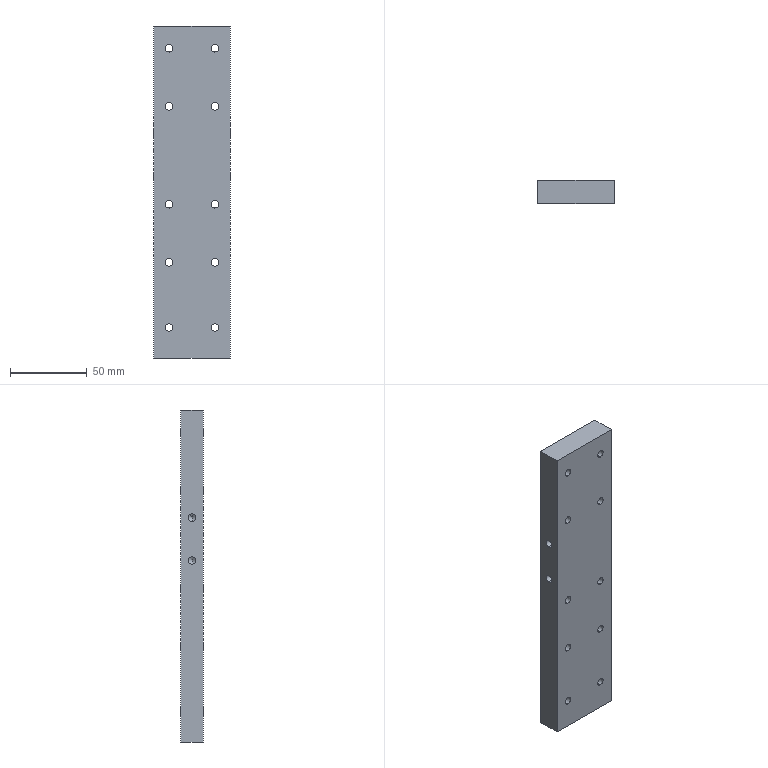Part | 1 solid | 50 faces | box 50 x 15 x 217 mm | volume 157448 mm3 | cylinder 32 | cone 12 | plane 6 | commonest cylinder face diameters 5 x28 6.8 x4
STEP:
#1=CARTESIAN_POINT('',(-11.6,7.5,-93.5));
#2=VERTEX_POINT('',#1);
#3=CARTESIAN_POINT('',(-18.4,7.5,-93.5));
#4=VERTEX_POINT('',#3);
#5=CARTESIAN_POINT('',(-15.,7.5,-93.5));
#6=DIRECTION('',(0.,0.,-1.));
#7=DIRECTION('',(-1.,0.,0.));
#8=AXIS2_PLACEMENT_3D('',#5,#6,#7);
#9=CIRCLE('',#8,3.4);
#10=EDGE_CURVE('',#2,#4,#9,.T.);
#11=ORIENTED_EDGE('',*,*,#10,.F.);
#12=CARTESIAN_POINT('',(-11.6,7.5,-108.5));
#13=VERTEX_POINT('',#12);
#14=CARTESIAN_POINT('',(-11.6,7.5,-108.5));
#15=DIRECTION('',(0.,0.,-1.));
#16=VECTOR('',#15,1000.);
#17=LINE('',#14,#16);
#18=EDGE_CURVE('',#2,#13,#17,.T.);
#19=ORIENTED_EDGE('',*,*,#18,.T.);
#20=CARTESIAN_POINT('',(-18.4,7.5,-108.5));
#21=VERTEX_POINT('',#20);
#22=CARTESIAN_POINT('',(-15.,7.5,-108.5));
#23=DIRECTION('',(0.,0.,-1.));
#24=DIRECTION('',(-1.,0.,0.));
#25=AXIS2_PLACEMENT_3D('',#22,#23,#24);
#26=CIRCLE('',#25,3.4);
#27=EDGE_CURVE('',#13,#21,#26,.T.);
#28=ORIENTED_EDGE('',*,*,#27,.T.);
#29=CARTESIAN_POINT('',(-18.4,7.5,-108.5));
#30=DIRECTION('',(0.,0.,-1.));
#31=VECTOR('',#30,1000.);
#32=LINE('',#29,#31);
#33=EDGE_CURVE('',#4,#21,#32,.T.);
#34=ORIENTED_EDGE('',*,*,#33,.F.);
#35=EDGE_LOOP('',(#11,#19,#28,#34));
#36=FACE_OUTER_BOUND('',#35,.T.);
#37=CARTESIAN_POINT('',(-15.,7.5,-108.5));
#38=DIRECTION('',(0.,0.,-1.));
#39=DIRECTION('',(-1.,0.,0.));
#40=AXIS2_PLACEMENT_3D('',#37,#38,#39);
#41=CYLINDRICAL_SURFACE('',#40,3.4);
#42=ADVANCED_FACE('',(#36),#41,.F.);
#43=CARTESIAN_POINT('',(-15.,7.5,-91.457));
#44=VERTEX_POINT('',#43);
#45=CARTESIAN_POINT('',(-18.4,7.5,-93.5));
#46=DIRECTION('',(-0.8572,0.,-0.515));
#47=VECTOR('',#46,1000.);
#48=LINE('',#45,#47);
#49=EDGE_CURVE('',#44,#4,#48,.T.);
#50=ORIENTED_EDGE('',*,*,#49,.F.);
#51=CARTESIAN_POINT('',(-11.6,7.5,-93.5));
#52=DIRECTION('',(0.8572,0.,-0.515));
#53=VECTOR('',#52,1000.);
#54=LINE('',#51,#53);
#55=EDGE_CURVE('',#44,#2,#54,.T.);
#56=ORIENTED_EDGE('',*,*,#55,.T.);
#57=ORIENTED_EDGE('',*,*,#10,.T.);
#58=EDGE_LOOP('',(#50,#56,#57));
#59=FACE_OUTER_BOUND('',#58,.T.);
#60=CARTESIAN_POINT('',(-15.,7.5,-93.5));
#61=DIRECTION('',(0.,0.,-1.));
#62=DIRECTION('',(-1.,0.,0.));
#63=AXIS2_PLACEMENT_3D('',#60,#61,#62);
#64=CONICAL_SURFACE('',#63,3.4,1.03);
#65=ADVANCED_FACE('',(#59),#64,.F.);
#66=CARTESIAN_POINT('',(18.4,7.5,-93.5));
#67=VERTEX_POINT('',#66);
#68=CARTESIAN_POINT('',(11.6,7.5,-93.5));
#69=VERTEX_POINT('',#68);
#70=CARTESIAN_POINT('',(15.,7.5,-93.5));
#71=DIRECTION('',(0.,0.,-1.));
#72=DIRECTION('',(-1.,0.,0.));
#73=AXIS2_PLACEMENT_3D('',#70,#71,#72);
#74=CIRCLE('',#73,3.4);
#75=EDGE_CURVE('',#67,#69,#74,.T.);
#76=ORIENTED_EDGE('',*,*,#75,.F.);
#77=CARTESIAN_POINT('',(18.4,7.5,-108.5));
#78=VERTEX_POINT('',#77);
#79=CARTESIAN_POINT('',(18.4,7.5,-108.5));
#80=DIRECTION('',(0.,0.,-1.));
#81=VECTOR('',#80,1000.);
#82=LINE('',#79,#81);
#83=EDGE_CURVE('',#67,#78,#82,.T.);
#84=ORIENTED_EDGE('',*,*,#83,.T.);
#85=CARTESIAN_POINT('',(11.6,7.5,-108.5));
#86=VERTEX_POINT('',#85);
#87=CARTESIAN_POINT('',(15.,7.5,-108.5));
#88=DIRECTION('',(0.,0.,-1.));
#89=DIRECTION('',(-1.,0.,0.));
#90=AXIS2_PLACEMENT_3D('',#87,#88,#89);
#91=CIRCLE('',#90,3.4);
#92=EDGE_CURVE('',#78,#86,#91,.T.);
#93=ORIENTED_EDGE('',*,*,#92,.T.);
#94=CARTESIAN_POINT('',(11.6,7.5,-108.5));
#95=DIRECTION('',(0.,0.,-1.));
#96=VECTOR('',#95,1000.);
#97=LINE('',#94,#96);
#98=EDGE_CURVE('',#69,#86,#97,.T.);
#99=ORIENTED_EDGE('',*,*,#98,.F.);
#100=EDGE_LOOP('',(#76,#84,#93,#99));
#101=FACE_OUTER_BOUND('',#100,.T.);
#102=CARTESIAN_POINT('',(15.,7.5,-108.5));
#103=DIRECTION('',(0.,0.,-1.));
#104=DIRECTION('',(-1.,0.,0.));
#105=AXIS2_PLACEMENT_3D('',#102,#103,#104);
#106=CYLINDRICAL_SURFACE('',#105,3.4);
#107=ADVANCED_FACE('',(#101),#106,.F.);
#108=CARTESIAN_POINT('',(15.,7.5,-91.457));
#109=VERTEX_POINT('',#108);
#110=CARTESIAN_POINT('',(11.6,7.5,-93.5));
#111=DIRECTION('',(-0.8572,0.,-0.515));
#112=VECTOR('',#111,1000.);
#113=LINE('',#110,#112);
#114=EDGE_CURVE('',#109,#69,#113,.T.);
#115=ORIENTED_EDGE('',*,*,#114,.F.);
#116=CARTESIAN_POINT('',(18.4,7.5,-93.5));
#117=DIRECTION('',(0.8572,0.,-0.515));
#118=VECTOR('',#117,1000.);
#119=LINE('',#116,#118);
#120=EDGE_CURVE('',#109,#67,#119,.T.);
#121=ORIENTED_EDGE('',*,*,#120,.T.);
#122=ORIENTED_EDGE('',*,*,#75,.T.);
#123=EDGE_LOOP('',(#115,#121,#122));
#124=FACE_OUTER_BOUND('',#123,.T.);
#125=CARTESIAN_POINT('',(15.,7.5,-93.5));
#126=DIRECTION('',(0.,0.,-1.));
#127=DIRECTION('',(-1.,0.,0.));
#128=AXIS2_PLACEMENT_3D('',#125,#126,#127);
#129=CONICAL_SURFACE('',#128,3.4,1.03);
#130=ADVANCED_FACE('',(#124),#129,.F.);
#131=CARTESIAN_POINT('',(-10.,7.5,7.6));
#132=VERTEX_POINT('',#131);
#133=CARTESIAN_POINT('',(-10.,7.5,12.6));
#134=VERTEX_POINT('',#133);
#135=CARTESIAN_POINT('',(-10.,7.5,10.1));
#136=DIRECTION('',(-1.,0.,0.));
#137=DIRECTION('',(0.,0.,1.));
#138=AXIS2_PLACEMENT_3D('',#135,#136,#137);
#139=CIRCLE('',#138,2.5);
#140=EDGE_CURVE('',#132,#134,#139,.T.);
#141=ORIENTED_EDGE('',*,*,#140,.F.);
#142=CARTESIAN_POINT('',(-25.,7.5,7.6));
#143=VERTEX_POINT('',#142);
#144=CARTESIAN_POINT('',(-25.,7.5,7.6));
#145=DIRECTION('',(-1.,0.,0.));
#146=VECTOR('',#145,1000.);
#147=LINE('',#144,#146);
#148=EDGE_CURVE('',#132,#143,#147,.T.);
#149=ORIENTED_EDGE('',*,*,#148,.T.);
#150=CARTESIAN_POINT('',(-25.,7.5,12.6));
#151=VERTEX_POINT('',#150);
#152=CARTESIAN_POINT('',(-25.,7.5,10.1));
#153=DIRECTION('',(-1.,0.,0.));
#154=DIRECTION('',(0.,0.,1.));
#155=AXIS2_PLACEMENT_3D('',#152,#153,#154);
#156=CIRCLE('',#155,2.5);
#157=EDGE_CURVE('',#143,#151,#156,.T.);
#158=ORIENTED_EDGE('',*,*,#157,.T.);
#159=CARTESIAN_POINT('',(-25.,7.5,12.6));
#160=DIRECTION('',(-1.,0.,0.));
#161=VECTOR('',#160,1000.);
#162=LINE('',#159,#161);
#163=EDGE_CURVE('',#134,#151,#162,.T.);
#164=ORIENTED_EDGE('',*,*,#163,.F.);
#165=EDGE_LOOP('',(#141,#149,#158,#164));
#166=FACE_OUTER_BOUND('',#165,.T.);
#167=CARTESIAN_POINT('',(-25.,7.5,10.1));
#168=DIRECTION('',(-1.,0.,0.));
#169=DIRECTION('',(0.,0.,1.));
#170=AXIS2_PLACEMENT_3D('',#167,#168,#169);
#171=CYLINDRICAL_SURFACE('',#170,2.5);
#172=ADVANCED_FACE('',(#166),#171,.F.);
#173=CARTESIAN_POINT('',(-8.498,7.5,10.1));
#174=VERTEX_POINT('',#173);
#175=CARTESIAN_POINT('',(-10.,7.5,12.6));
#176=DIRECTION('',(-0.515,0.,0.8572));
#177=VECTOR('',#176,1000.);
#178=LINE('',#175,#177);
#179=EDGE_CURVE('',#174,#134,#178,.T.);
#180=ORIENTED_EDGE('',*,*,#179,.F.);
#181=CARTESIAN_POINT('',(-10.,7.5,7.6));
#182=DIRECTION('',(-0.515,0.,-0.8572));
#183=VECTOR('',#182,1000.);
#184=LINE('',#181,#183);
#185=EDGE_CURVE('',#174,#132,#184,.T.);
#186=ORIENTED_EDGE('',*,*,#185,.T.);
#187=ORIENTED_EDGE('',*,*,#140,.T.);
#188=EDGE_LOOP('',(#180,#186,#187));
#189=FACE_OUTER_BOUND('',#188,.T.);
#190=CARTESIAN_POINT('',(-10.,7.5,10.1));
#191=DIRECTION('',(-1.,0.,0.));
#192=DIRECTION('',(0.,0.,1.));
#193=AXIS2_PLACEMENT_3D('',#190,#191,#192);
#194=CONICAL_SURFACE('',#193,2.5,1.03);
#195=ADVANCED_FACE('',(#189),#194,.F.);
#196=CARTESIAN_POINT('',(-10.,7.5,35.6));
#197=VERTEX_POINT('',#196);
#198=CARTESIAN_POINT('',(-10.,7.5,40.6));
#199=VERTEX_POINT('',#198);
#200=CARTESIAN_POINT('',(-10.,7.5,38.1));
#201=DIRECTION('',(-1.,0.,0.));
#202=DIRECTION('',(0.,0.,1.));
#203=AXIS2_PLACEMENT_3D('',#200,#201,#202);
#204=CIRCLE('',#203,2.5);
#205=EDGE_CURVE('',#197,#199,#204,.T.);
#206=ORIENTED_EDGE('',*,*,#205,.F.);
#207=CARTESIAN_POINT('',(-25.,7.5,35.6));
#208=VERTEX_POINT('',#207);
#209=CARTESIAN_POINT('',(-25.,7.5,35.6));
#210=DIRECTION('',(-1.,0.,0.));
#211=VECTOR('',#210,1000.);
#212=LINE('',#209,#211);
#213=EDGE_CURVE('',#197,#208,#212,.T.);
#214=ORIENTED_EDGE('',*,*,#213,.T.);
#215=CARTESIAN_POINT('',(-25.,7.5,40.6));
#216=VERTEX_POINT('',#215);
#217=CARTESIAN_POINT('',(-25.,7.5,38.1));
#218=DIRECTION('',(-1.,0.,0.));
#219=DIRECTION('',(0.,0.,1.));
#220=AXIS2_PLACEMENT_3D('',#217,#218,#219);
#221=CIRCLE('',#220,2.5);
#222=EDGE_CURVE('',#208,#216,#221,.T.);
#223=ORIENTED_EDGE('',*,*,#222,.T.);
#224=CARTESIAN_POINT('',(-25.,7.5,40.6));
#225=DIRECTION('',(-1.,0.,0.));
#226=VECTOR('',#225,1000.);
#227=LINE('',#224,#226);
#228=EDGE_CURVE('',#199,#216,#227,.T.);
#229=ORIENTED_EDGE('',*,*,#228,.F.);
#230=EDGE_LOOP('',(#206,#214,#223,#229));
#231=FACE_OUTER_BOUND('',#230,.T.);
#232=CARTESIAN_POINT('',(-25.,7.5,38.1));
#233=DIRECTION('',(-1.,0.,0.));
#234=DIRECTION('',(0.,0.,1.));
#235=AXIS2_PLACEMENT_3D('',#232,#233,#234);
#236=CYLINDRICAL_SURFACE('',#235,2.5);
#237=ADVANCED_FACE('',(#231),#236,.F.);
#238=CARTESIAN_POINT('',(-8.498,7.5,38.1));
#239=VERTEX_POINT('',#238);
#240=CARTESIAN_POINT('',(-10.,7.5,40.6));
#241=DIRECTION('',(-0.515,0.,0.8572));
#242=VECTOR('',#241,1000.);
#243=LINE('',#240,#242);
#244=EDGE_CURVE('',#239,#199,#243,.T.);
#245=ORIENTED_EDGE('',*,*,#244,.F.);
#246=CARTESIAN_POINT('',(-10.,7.5,35.6));
#247=DIRECTION('',(-0.515,0.,-0.8572));
#248=VECTOR('',#247,1000.);
#249=LINE('',#246,#248);
#250=EDGE_CURVE('',#239,#197,#249,.T.);
#251=ORIENTED_EDGE('',*,*,#250,.T.);
#252=ORIENTED_EDGE('',*,*,#205,.T.);
#253=EDGE_LOOP('',(#245,#251,#252));
#254=FACE_OUTER_BOUND('',#253,.T.);
#255=CARTESIAN_POINT('',(-10.,7.5,38.1));
#256=DIRECTION('',(-1.,0.,0.));
#257=DIRECTION('',(0.,0.,1.));
#258=AXIS2_PLACEMENT_3D('',#255,#256,#257);
#259=CONICAL_SURFACE('',#258,2.5,1.03);
#260=ADVANCED_FACE('',(#254),#259,.F.);
#261=CARTESIAN_POINT('',(10.,7.5,12.6));
#262=VERTEX_POINT('',#261);
#263=CARTESIAN_POINT('',(10.,7.5,7.6));
#264=VERTEX_POINT('',#263);
#265=CARTESIAN_POINT('',(10.,7.5,10.1));
#266=DIRECTION('',(1.,0.,0.));
#267=DIRECTION('',(0.,0.,-1.));
#268=AXIS2_PLACEMENT_3D('',#265,#266,#267);
#269=CIRCLE('',#268,2.5);
#270=EDGE_CURVE('',#262,#264,#269,.T.);
#271=ORIENTED_EDGE('',*,*,#270,.F.);
#272=CARTESIAN_POINT('',(25.,7.5,12.6));
#273=VERTEX_POINT('',#272);
#274=CARTESIAN_POINT('',(25.,7.5,12.6));
#275=DIRECTION('',(1.,0.,0.));
#276=VECTOR('',#275,1000.);
#277=LINE('',#274,#276);
#278=EDGE_CURVE('',#262,#273,#277,.T.);
#279=ORIENTED_EDGE('',*,*,#278,.T.);
#280=CARTESIAN_POINT('',(25.,7.5,7.6));
#281=VERTEX_POINT('',#280);
#282=CARTESIAN_POINT('',(25.,7.5,10.1));
#283=DIRECTION('',(1.,0.,0.));
#284=DIRECTION('',(0.,0.,-1.));
#285=AXIS2_PLACEMENT_3D('',#282,#283,#284);
#286=CIRCLE('',#285,2.5);
#287=EDGE_CURVE('',#273,#281,#286,.T.);
#288=ORIENTED_EDGE('',*,*,#287,.T.);
#289=CARTESIAN_POINT('',(25.,7.5,7.6));
#290=DIRECTION('',(1.,0.,0.));
#291=VECTOR('',#290,1000.);
#292=LINE('',#289,#291);
#293=EDGE_CURVE('',#264,#281,#292,.T.);
#294=ORIENTED_EDGE('',*,*,#293,.F.);
#295=EDGE_LOOP('',(#271,#279,#288,#294));
#296=FACE_OUTER_BOUND('',#295,.T.);
#297=CARTESIAN_POINT('',(25.,7.5,10.1));
#298=DIRECTION('',(1.,0.,0.));
#299=DIRECTION('',(0.,0.,-1.));
#300=AXIS2_PLACEMENT_3D('',#297,#298,#299);
#301=CYLINDRICAL_SURFACE('',#300,2.5);
#302=ADVANCED_FACE('',(#296),#301,.F.);
#303=CARTESIAN_POINT('',(8.498,7.5,10.1));
#304=VERTEX_POINT('',#303);
#305=CARTESIAN_POINT('',(10.,7.5,7.6));
#306=DIRECTION('',(0.515,0.,-0.8572));
#307=VECTOR('',#306,1000.);
#308=LINE('',#305,#307);
#309=EDGE_CURVE('',#304,#264,#308,.T.);
#310=ORIENTED_EDGE('',*,*,#309,.F.);
#311=CARTESIAN_POINT('',(10.,7.5,12.6));
#312=DIRECTION('',(0.515,0.,0.8572));
#313=VECTOR('',#312,1000.);
#314=LINE('',#311,#313);
#315=EDGE_CURVE('',#304,#262,#314,.T.);
#316=ORIENTED_EDGE('',*,*,#315,.T.);
#317=ORIENTED_EDGE('',*,*,#270,.T.);
#318=EDGE_LOOP('',(#310,#316,#317));
#319=FACE_OUTER_BOUND('',#318,.T.);
#320=CARTESIAN_POINT('',(10.,7.5,10.1));
#321=DIRECTION('',(1.,0.,0.));
#322=DIRECTION('',(0.,0.,-1.));
#323=AXIS2_PLACEMENT_3D('',#320,#321,#322);
#324=CONICAL_SURFACE('',#323,2.5,1.03);
#325=ADVANCED_FACE('',(#319),#324,.F.);
#326=CARTESIAN_POINT('',(10.,7.5,40.6));
#327=VERTEX_POINT('',#326);
#328=CARTESIAN_POINT('',(10.,7.5,35.6));
#329=VERTEX_POINT('',#328);
#330=CARTESIAN_POINT('',(10.,7.5,38.1));
#331=DIRECTION('',(1.,0.,0.));
#332=DIRECTION('',(0.,0.,-1.));
#333=AXIS2_PLACEMENT_3D('',#330,#331,#332);
#334=CIRCLE('',#333,2.5);
#335=EDGE_CURVE('',#327,#329,#334,.T.);
#336=ORIENTED_EDGE('',*,*,#335,.F.);
#337=CARTESIAN_POINT('',(25.,7.5,40.6));
#338=VERTEX_POINT('',#337);
#339=CARTESIAN_POINT('',(25.,7.5,40.6));
#340=DIRECTION('',(1.,0.,0.));
#341=VECTOR('',#340,1000.);
#342=LINE('',#339,#341);
#343=EDGE_CURVE('',#327,#338,#342,.T.);
#344=ORIENTED_EDGE('',*,*,#343,.T.);
#345=CARTESIAN_POINT('',(25.,7.5,35.6));
#346=VERTEX_POINT('',#345);
#347=CARTESIAN_POINT('',(25.,7.5,38.1));
#348=DIRECTION('',(1.,0.,0.));
#349=DIRECTION('',(0.,0.,-1.));
#350=AXIS2_PLACEMENT_3D('',#347,#348,#349);
#351=CIRCLE('',#350,2.5);
#352=EDGE_CURVE('',#338,#346,#351,.T.);
#353=ORIENTED_EDGE('',*,*,#352,.T.);
#354=CARTESIAN_POINT('',(25.,7.5,35.6));
#355=DIRECTION('',(1.,0.,0.));
#356=VECTOR('',#355,1000.);
#357=LINE('',#354,#356);
#358=EDGE_CURVE('',#329,#346,#357,.T.);
#359=ORIENTED_EDGE('',*,*,#358,.F.);
#360=EDGE_LOOP('',(#336,#344,#353,#359));
#361=FACE_OUTER_BOUND('',#360,.T.);
#362=CARTESIAN_POINT('',(25.,7.5,38.1));
#363=DIRECTION('',(1.,0.,0.));
#364=DIRECTION('',(0.,0.,-1.));
#365=AXIS2_PLACEMENT_3D('',#362,#363,#364);
#366=CYLINDRICAL_SURFACE('',#365,2.5);
#367=ADVANCED_FACE('',(#361),#366,.F.);
#368=CARTESIAN_POINT('',(8.498,7.5,38.1));
#369=VERTEX_POINT('',#368);
#370=CARTESIAN_POINT('',(10.,7.5,35.6));
#371=DIRECTION('',(0.515,0.,-0.8572));
#372=VECTOR('',#371,1000.);
#373=LINE('',#370,#372);
#374=EDGE_CURVE('',#369,#329,#373,.T.);
#375=ORIENTED_EDGE('',*,*,#374,.F.);
#376=CARTESIAN_POINT('',(10.,7.5,40.6));
#377=DIRECTION('',(0.515,0.,0.8572));
#378=VECTOR('',#377,1000.);
#379=LINE('',#376,#378);
#380=EDGE_CURVE('',#369,#327,#379,.T.);
#381=ORIENTED_EDGE('',*,*,#380,.T.);
#382=ORIENTED_EDGE('',*,*,#335,.T.);
#383=EDGE_LOOP('',(#375,#381,#382));
#384=FACE_OUTER_BOUND('',#383,.T.);
#385=CARTESIAN_POINT('',(10.,7.5,38.1));
#386=DIRECTION('',(1.,0.,0.));
#387=DIRECTION('',(0.,0.,-1.));
#388=AXIS2_PLACEMENT_3D('',#385,#386,#387);
#389=CONICAL_SURFACE('',#388,2.5,1.03);
#390=ADVANCED_FACE('',(#384),#389,.F.);
#391=CARTESIAN_POINT('',(-15.,0.,-91.));
#392=VERTEX_POINT('',#391);
#393=CARTESIAN_POINT('',(-15.,0.,-86.));
#394=VERTEX_POINT('',#393);
#395=CARTESIAN_POINT('',(-15.,0.,-88.5));
#396=DIRECTION('',(0.,1.,0.));
#397=DIRECTION('',(0.,0.,1.));
#398=AXIS2_PLACEMENT_3D('',#395,#396,#397);
#399=CIRCLE('',#398,2.5);
#400=EDGE_CURVE('',#392,#394,#399,.T.);
#401=ORIENTED_EDGE('',*,*,#400,.F.);
#402=CARTESIAN_POINT('',(-15.,15.,-91.));
#403=VERTEX_POINT('',#402);
#404=CARTESIAN_POINT('',(-15.,15.,-91.));
#405=DIRECTION('',(0.,1.,0.));
#406=VECTOR('',#405,1000.);
#407=LINE('',#404,#406);
#408=EDGE_CURVE('',#392,#403,#407,.T.);
#409=ORIENTED_EDGE('',*,*,#408,.T.);
#410=CARTESIAN_POINT('',(-15.,15.,-86.));
#411=VERTEX_POINT('',#410);
#412=CARTESIAN_POINT('',(-15.,15.,-88.5));
#413=DIRECTION('',(0.,1.,0.));
#414=DIRECTION('',(0.,0.,1.));
#415=AXIS2_PLACEMENT_3D('',#412,#413,#414);
#416=CIRCLE('',#415,2.5);
#417=EDGE_CURVE('',#403,#411,#416,.T.);
#418=ORIENTED_EDGE('',*,*,#417,.T.);
#419=CARTESIAN_POINT('',(-15.,15.,-86.));
#420=DIRECTION('',(0.,1.,0.));
#421=VECTOR('',#420,1000.);
#422=LINE('',#419,#421);
#423=EDGE_CURVE('',#394,#411,#422,.T.);
#424=ORIENTED_EDGE('',*,*,#423,.F.);
#425=EDGE_LOOP('',(#401,#409,#418,#424));
#426=FACE_OUTER_BOUND('',#425,.T.);
#427=CARTESIAN_POINT('',(-15.,15.,-88.5));
#428=DIRECTION('',(0.,1.,0.));
#429=DIRECTION('',(0.,0.,1.));
#430=AXIS2_PLACEMENT_3D('',#427,#428,#429);
#431=CYLINDRICAL_SURFACE('',#430,2.5);
#432=ADVANCED_FACE('',(#426),#431,.F.);
#433=CARTESIAN_POINT('',(15.,0.,-91.));
#434=VERTEX_POINT('',#433);
#435=CARTESIAN_POINT('',(15.,0.,-86.));
#436=VERTEX_POINT('',#435);
#437=CARTESIAN_POINT('',(15.,0.,-88.5));
#438=DIRECTION('',(0.,1.,0.));
#439=DIRECTION('',(0.,0.,1.));
#440=AXIS2_PLACEMENT_3D('',#437,#438,#439);
#441=CIRCLE('',#440,2.5);
#442=EDGE_CURVE('',#434,#436,#441,.T.);
#443=ORIENTED_EDGE('',*,*,#442,.F.);
#444=CARTESIAN_POINT('',(15.,15.,-91.));
#445=VERTEX_POINT('',#444);
#446=CARTESIAN_POINT('',(15.,15.,-91.));
#447=DIRECTION('',(0.,1.,0.));
#448=VECTOR('',#447,1000.);
#449=LINE('',#446,#448);
#450=EDGE_CURVE('',#434,#445,#449,.T.);
#451=ORIENTED_EDGE('',*,*,#450,.T.);
#452=CARTESIAN_POINT('',(15.,15.,-86.));
#453=VERTEX_POINT('',#452);
#454=CARTESIAN_POINT('',(15.,15.,-88.5));
#455=DIRECTION('',(0.,1.,0.));
#456=DIRECTION('',(0.,0.,1.));
#457=AXIS2_PLACEMENT_3D('',#454,#455,#456);
#458=CIRCLE('',#457,2.5);
#459=EDGE_CURVE('',#445,#453,#458,.T.);
#460=ORIENTED_EDGE('',*,*,#459,.T.);
#461=CARTESIAN_POINT('',(15.,15.,-86.));
#462=DIRECTION('',(0.,1.,0.));
#463=VECTOR('',#462,1000.);
#464=LINE('',#461,#463);
#465=EDGE_CURVE('',#436,#453,#464,.T.);
#466=ORIENTED_EDGE('',*,*,#465,.F.);
#467=EDGE_LOOP('',(#443,#451,#460,#466));
#468=FACE_OUTER_BOUND('',#467,.T.);
#469=CARTESIAN_POINT('',(15.,15.,-88.5));
#470=DIRECTION('',(0.,1.,0.));
#471=DIRECTION('',(0.,0.,1.));
#472=AXIS2_PLACEMENT_3D('',#469,#470,#471);
#473=CYLINDRICAL_SURFACE('',#472,2.5);
#474=ADVANCED_FACE('',(#468),#473,.F.);
#475=CARTESIAN_POINT('',(-15.,0.,96.5));
#476=VERTEX_POINT('',#475);
#477=CARTESIAN_POINT('',(-15.,0.,91.5));
#478=VERTEX_POINT('',#477);
#479=CARTESIAN_POINT('',(-15.,0.,94.));
#480=DIRECTION('',(0.,-1.,0.));
#481=DIRECTION('',(0.,0.,-1.));
#482=AXIS2_PLACEMENT_3D('',#479,#480,#481);
#483=CIRCLE('',#482,2.5);
#484=EDGE_CURVE('',#476,#478,#483,.T.);
#485=ORIENTED_EDGE('',*,*,#484,.T.);
#486=CARTESIAN_POINT('',(-15.,15.,91.5));
#487=VERTEX_POINT('',#486);
#488=CARTESIAN_POINT('',(-15.,15.,91.5));
#489=DIRECTION('',(0.,1.,0.));
#490=VECTOR('',#489,1000.);
#491=LINE('',#488,#490);
#492=EDGE_CURVE('',#478,#487,#491,.T.);
#493=ORIENTED_EDGE('',*,*,#492,.T.);
#494=CARTESIAN_POINT('',(-15.,15.,96.5));
#495=VERTEX_POINT('',#494);
#496=CARTESIAN_POINT('',(-15.,15.,94.));
#497=DIRECTION('',(0.,1.,0.));
#498=DIRECTION('',(0.,0.,1.));
#499=AXIS2_PLACEMENT_3D('',#496,#497,#498);
#500=CIRCLE('',#499,2.5);
#501=EDGE_CURVE('',#487,#495,#500,.T.);
#502=ORIENTED_EDGE('',*,*,#501,.T.);
#503=CARTESIAN_POINT('',(-15.,15.,96.5));
#504=DIRECTION('',(0.,1.,0.));
#505=VECTOR('',#504,1000.);
#506=LINE('',#503,#505);
#507=EDGE_CURVE('',#476,#495,#506,.T.);
#508=ORIENTED_EDGE('',*,*,#507,.F.);
#509=EDGE_LOOP('',(#485,#493,#502,#508));
#510=FACE_OUTER_BOUND('',#509,.T.);
#511=CARTESIAN_POINT('',(-15.,15.,94.));
#512=DIRECTION('',(0.,1.,0.));
#513=DIRECTION('',(0.,0.,1.));
#514=AXIS2_PLACEMENT_3D('',#511,#512,#513);
#515=CYLINDRICAL_SURFACE('',#514,2.5);
#516=ADVANCED_FACE('',(#510),#515,.F.);
#517=CARTESIAN_POINT('',(15.,0.,96.5));
#518=VERTEX_POINT('',#517);
#519=CARTESIAN_POINT('',(15.,0.,91.5));
#520=VERTEX_POINT('',#519);
#521=CARTESIAN_POINT('',(15.,0.,94.));
#522=DIRECTION('',(0.,-1.,0.));
#523=DIRECTION('',(0.,0.,-1.));
#524=AXIS2_PLACEMENT_3D('',#521,#522,#523);
#525=CIRCLE('',#524,2.5);
#526=EDGE_CURVE('',#518,#520,#525,.T.);
#527=ORIENTED_EDGE('',*,*,#526,.T.);
#528=CARTESIAN_POINT('',(15.,15.,91.5));
#529=VERTEX_POINT('',#528);
#530=CARTESIAN_POINT('',(15.,15.,91.5));
#531=DIRECTION('',(0.,1.,0.));
#532=VECTOR('',#531,1000.);
#533=LINE('',#530,#532);
#534=EDGE_CURVE('',#520,#529,#533,.T.);
#535=ORIENTED_EDGE('',*,*,#534,.T.);
#536=CARTESIAN_POINT('',(15.,15.,96.5));
#537=VERTEX_POINT('',#536);
#538=CARTESIAN_POINT('',(15.,15.,94.));
#539=DIRECTION('',(0.,1.,0.));
#540=DIRECTION('',(0.,0.,1.));
#541=AXIS2_PLACEMENT_3D('',#538,#539,#540);
#542=CIRCLE('',#541,2.5);
#543=EDGE_CURVE('',#529,#537,#542,.T.);
#544=ORIENTED_EDGE('',*,*,#543,.T.);
#545=CARTESIAN_POINT('',(15.,15.,96.5));
#546=DIRECTION('',(0.,1.,0.));
#547=VECTOR('',#546,1000.);
#548=LINE('',#545,#547);
#549=EDGE_CURVE('',#518,#537,#548,.T.);
#550=ORIENTED_EDGE('',*,*,#549,.F.);
#551=EDGE_LOOP('',(#527,#535,#544,#550));
#552=FACE_OUTER_BOUND('',#551,.T.);
#553=CARTESIAN_POINT('',(15.,15.,94.));
#554=DIRECTION('',(0.,1.,0.));
#555=DIRECTION('',(0.,0.,1.));
#556=AXIS2_PLACEMENT_3D('',#553,#554,#555);
#557=CYLINDRICAL_SURFACE('',#556,2.5);
#558=ADVANCED_FACE('',(#552),#557,.F.);
#559=CARTESIAN_POINT('',(-15.,0.,58.5));
#560=VERTEX_POINT('',#559);
#561=CARTESIAN_POINT('',(-15.,0.,53.5));
#562=VERTEX_POINT('',#561);
#563=CARTESIAN_POINT('',(-15.,0.,56.));
#564=DIRECTION('',(0.,-1.,0.));
#565=DIRECTION('',(0.,0.,-1.));
#566=AXIS2_PLACEMENT_3D('',#563,#564,#565);
#567=CIRCLE('',#566,2.5);
#568=EDGE_CURVE('',#560,#562,#567,.T.);
#569=ORIENTED_EDGE('',*,*,#568,.T.);
#570=CARTESIAN_POINT('',(-15.,15.,53.5));
#571=VERTEX_POINT('',#570);
#572=CARTESIAN_POINT('',(-15.,15.,53.5));
#573=DIRECTION('',(0.,1.,0.));
#574=VECTOR('',#573,1000.);
#575=LINE('',#572,#574);
#576=EDGE_CURVE('',#562,#571,#575,.T.);
#577=ORIENTED_EDGE('',*,*,#576,.T.);
#578=CARTESIAN_POINT('',(-15.,15.,58.5));
#579=VERTEX_POINT('',#578);
#580=CARTESIAN_POINT('',(-15.,15.,56.));
#581=DIRECTION('',(0.,1.,0.));
#582=DIRECTION('',(0.,0.,1.));
#583=AXIS2_PLACEMENT_3D('',#580,#581,#582);
#584=CIRCLE('',#583,2.5);
#585=EDGE_CURVE('',#571,#579,#584,.T.);
#586=ORIENTED_EDGE('',*,*,#585,.T.);
#587=CARTESIAN_POINT('',(-15.,15.,58.5));
#588=DIRECTION('',(0.,1.,0.));
#589=VECTOR('',#588,1000.);
#590=LINE('',#587,#589);
#591=EDGE_CURVE('',#560,#579,#590,.T.);
#592=ORIENTED_EDGE('',*,*,#591,.F.);
#593=EDGE_LOOP('',(#569,#577,#586,#592));
#594=FACE_OUTER_BOUND('',#593,.T.);
#595=CARTESIAN_POINT('',(-15.,15.,56.));
#596=DIRECTION('',(0.,1.,0.));
#597=DIRECTION('',(0.,0.,1.));
#598=AXIS2_PLACEMENT_3D('',#595,#596,#597);
#599=CYLINDRICAL_SURFACE('',#598,2.5);
#600=ADVANCED_FACE('',(#594),#599,.F.);
#601=CARTESIAN_POINT('',(15.,0.,58.5));
#602=VERTEX_POINT('',#601);
#603=CARTESIAN_POINT('',(15.,0.,53.5));
#604=VERTEX_POINT('',#603);
#605=CARTESIAN_POINT('',(15.,0.,56.));
#606=DIRECTION('',(0.,-1.,0.));
#607=DIRECTION('',(0.,0.,-1.));
#608=AXIS2_PLACEMENT_3D('',#605,#606,#607);
#609=CIRCLE('',#608,2.5);
#610=EDGE_CURVE('',#602,#604,#609,.T.);
#611=ORIENTED_EDGE('',*,*,#610,.T.);
#612=CARTESIAN_POINT('',(15.,15.,53.5));
#613=VERTEX_POINT('',#612);
#614=CARTESIAN_POINT('',(15.,15.,53.5));
#615=DIRECTION('',(0.,1.,0.));
#616=VECTOR('',#615,1000.);
#617=LINE('',#614,#616);
#618=EDGE_CURVE('',#604,#613,#617,.T.);
#619=ORIENTED_EDGE('',*,*,#618,.T.);
#620=CARTESIAN_POINT('',(15.,15.,58.5));
#621=VERTEX_POINT('',#620);
#622=CARTESIAN_POINT('',(15.,15.,56.));
#623=DIRECTION('',(0.,1.,0.));
#624=DIRECTION('',(0.,0.,1.));
#625=AXIS2_PLACEMENT_3D('',#622,#623,#624);
#626=CIRCLE('',#625,2.5);
#627=EDGE_CURVE('',#613,#621,#626,.T.);
#628=ORIENTED_EDGE('',*,*,#627,.T.);
#629=CARTESIAN_POINT('',(15.,15.,58.5));
#630=DIRECTION('',(0.,1.,0.));
#631=VECTOR('',#630,1000.);
#632=LINE('',#629,#631);
#633=EDGE_CURVE('',#602,#621,#632,.T.);
#634=ORIENTED_EDGE('',*,*,#633,.F.);
#635=EDGE_LOOP('',(#611,#619,#628,#634));
#636=FACE_OUTER_BOUND('',#635,.T.);
#637=CARTESIAN_POINT('',(15.,15.,56.));
#638=DIRECTION('',(0.,1.,0.));
#639=DIRECTION('',(0.,0.,1.));
#640=AXIS2_PLACEMENT_3D('',#637,#638,#639);
#641=CYLINDRICAL_SURFACE('',#640,2.5);
#642=ADVANCED_FACE('',(#636),#641,.F.);
#643=CARTESIAN_POINT('',(15.,0.,-5.5));
#644=VERTEX_POINT('',#643);
#645=CARTESIAN_POINT('',(15.,0.,-10.5));
#646=VERTEX_POINT('',#645);
#647=CARTESIAN_POINT('',(15.,0.,-8.));
#648=DIRECTION('',(0.,-1.,0.));
#649=DIRECTION('',(0.,0.,-1.));
#650=AXIS2_PLACEMENT_3D('',#647,#648,#649);
#651=CIRCLE('',#650,2.5);
#652=EDGE_CURVE('',#644,#646,#651,.T.);
#653=ORIENTED_EDGE('',*,*,#652,.T.);
#654=CARTESIAN_POINT('',(15.,15.,-10.5));
#655=VERTEX_POINT('',#654);
#656=CARTESIAN_POINT('',(15.,15.,-10.5));
#657=DIRECTION('',(0.,1.,0.));
#658=VECTOR('',#657,1000.);
#659=LINE('',#656,#658);
#660=EDGE_CURVE('',#646,#655,#659,.T.);
#661=ORIENTED_EDGE('',*,*,#660,.T.);
#662=CARTESIAN_POINT('',(15.,15.,-5.5));
#663=VERTEX_POINT('',#662);
#664=CARTESIAN_POINT('',(15.,15.,-8.));
#665=DIRECTION('',(0.,1.,0.));
#666=DIRECTION('',(0.,0.,1.));
#667=AXIS2_PLACEMENT_3D('',#664,#665,#666);
#668=CIRCLE('',#667,2.5);
#669=EDGE_CURVE('',#655,#663,#668,.T.);
#670=ORIENTED_EDGE('',*,*,#669,.T.);
#671=CARTESIAN_POINT('',(15.,15.,-5.5));
#672=DIRECTION('',(0.,1.,0.));
#673=VECTOR('',#672,1000.);
#674=LINE('',#671,#673);
#675=EDGE_CURVE('',#644,#663,#674,.T.);
#676=ORIENTED_EDGE('',*,*,#675,.F.);
#677=EDGE_LOOP('',(#653,#661,#670,#676));
#678=FACE_OUTER_BOUND('',#677,.T.);
#679=CARTESIAN_POINT('',(15.,15.,-8.));
#680=DIRECTION('',(0.,1.,0.));
#681=DIRECTION('',(0.,0.,1.));
#682=AXIS2_PLACEMENT_3D('',#679,#680,#681);
#683=CYLINDRICAL_SURFACE('',#682,2.5);
#684=ADVANCED_FACE('',(#678),#683,.F.);
#685=CARTESIAN_POINT('',(-15.,0.,-5.5));
#686=VERTEX_POINT('',#685);
#687=CARTESIAN_POINT('',(-15.,0.,-10.5));
#688=VERTEX_POINT('',#687);
#689=CARTESIAN_POINT('',(-15.,0.,-8.));
#690=DIRECTION('',(0.,-1.,0.));
#691=DIRECTION('',(0.,0.,-1.));
#692=AXIS2_PLACEMENT_3D('',#689,#690,#691);
#693=CIRCLE('',#692,2.5);
#694=EDGE_CURVE('',#686,#688,#693,.T.);
#695=ORIENTED_EDGE('',*,*,#694,.T.);
#696=CARTESIAN_POINT('',(-15.,15.,-10.5));
#697=VERTEX_POINT('',#696);
#698=CARTESIAN_POINT('',(-15.,15.,-10.5));
#699=DIRECTION('',(0.,1.,0.));
#700=VECTOR('',#699,1000.);
#701=LINE('',#698,#700);
#702=EDGE_CURVE('',#688,#697,#701,.T.);
#703=ORIENTED_EDGE('',*,*,#702,.T.);
#704=CARTESIAN_POINT('',(-15.,15.,-5.5));
#705=VERTEX_POINT('',#704);
#706=CARTESIAN_POINT('',(-15.,15.,-8.));
#707=DIRECTION('',(0.,1.,0.));
#708=DIRECTION('',(0.,0.,1.));
#709=AXIS2_PLACEMENT_3D('',#706,#707,#708);
#710=CIRCLE('',#709,2.5);
#711=EDGE_CURVE('',#697,#705,#710,.T.);
#712=ORIENTED_EDGE('',*,*,#711,.T.);
#713=CARTESIAN_POINT('',(-15.,15.,-5.5));
#714=DIRECTION('',(0.,1.,0.));
#715=VECTOR('',#714,1000.);
#716=LINE('',#713,#715);
#717=EDGE_CURVE('',#686,#705,#716,.T.);
#718=ORIENTED_EDGE('',*,*,#717,.F.);
#719=EDGE_LOOP('',(#695,#703,#712,#718));
#720=FACE_OUTER_BOUND('',#719,.T.);
#721=CARTESIAN_POINT('',(-15.,15.,-8.));
#722=DIRECTION('',(0.,1.,0.));
#723=DIRECTION('',(0.,0.,1.));
#724=AXIS2_PLACEMENT_3D('',#721,#722,#723);
#725=CYLINDRICAL_SURFACE('',#724,2.5);
#726=ADVANCED_FACE('',(#720),#725,.F.);
#727=CARTESIAN_POINT('',(-15.,0.,-43.5));
#728=VERTEX_POINT('',#727);
#729=CARTESIAN_POINT('',(-15.,0.,-48.5));
#730=VERTEX_POINT('',#729);
#731=CARTESIAN_POINT('',(-15.,0.,-46.));
#732=DIRECTION('',(0.,-1.,0.));
#733=DIRECTION('',(0.,0.,-1.));
#734=AXIS2_PLACEMENT_3D('',#731,#732,#733);
#735=CIRCLE('',#734,2.5);
#736=EDGE_CURVE('',#728,#730,#735,.T.);
#737=ORIENTED_EDGE('',*,*,#736,.T.);
#738=CARTESIAN_POINT('',(-15.,15.,-48.5));
#739=VERTEX_POINT('',#738);
#740=CARTESIAN_POINT('',(-15.,15.,-48.5));
#741=DIRECTION('',(0.,1.,0.));
#742=VECTOR('',#741,1000.);
#743=LINE('',#740,#742);
#744=EDGE_CURVE('',#730,#739,#743,.T.);
#745=ORIENTED_EDGE('',*,*,#744,.T.);
#746=CARTESIAN_POINT('',(-15.,15.,-43.5));
#747=VERTEX_POINT('',#746);
#748=CARTESIAN_POINT('',(-15.,15.,-46.));
#749=DIRECTION('',(0.,1.,0.));
#750=DIRECTION('',(0.,0.,1.));
#751=AXIS2_PLACEMENT_3D('',#748,#749,#750);
#752=CIRCLE('',#751,2.5);
#753=EDGE_CURVE('',#739,#747,#752,.T.);
#754=ORIENTED_EDGE('',*,*,#753,.T.);
#755=CARTESIAN_POINT('',(-15.,15.,-43.5));
#756=DIRECTION('',(0.,1.,0.));
#757=VECTOR('',#756,1000.);
#758=LINE('',#755,#757);
#759=EDGE_CURVE('',#728,#747,#758,.T.);
#760=ORIENTED_EDGE('',*,*,#759,.F.);
#761=EDGE_LOOP('',(#737,#745,#754,#760));
#762=FACE_OUTER_BOUND('',#761,.T.);
#763=CARTESIAN_POINT('',(-15.,15.,-46.));
#764=DIRECTION('',(0.,1.,0.));
#765=DIRECTION('',(0.,0.,1.));
#766=AXIS2_PLACEMENT_3D('',#763,#764,#765);
#767=CYLINDRICAL_SURFACE('',#766,2.5);
#768=ADVANCED_FACE('',(#762),#767,.F.);
#769=CARTESIAN_POINT('',(15.,0.,-43.5));
#770=VERTEX_POINT('',#769);
#771=CARTESIAN_POINT('',(15.,0.,-48.5));
#772=VERTEX_POINT('',#771);
#773=CARTESIAN_POINT('',(15.,0.,-46.));
#774=DIRECTION('',(0.,-1.,0.));
#775=DIRECTION('',(0.,0.,-1.));
#776=AXIS2_PLACEMENT_3D('',#773,#774,#775);
#777=CIRCLE('',#776,2.5);
#778=EDGE_CURVE('',#770,#772,#777,.T.);
#779=ORIENTED_EDGE('',*,*,#778,.T.);
#780=CARTESIAN_POINT('',(15.,15.,-48.5));
#781=VERTEX_POINT('',#780);
#782=CARTESIAN_POINT('',(15.,15.,-48.5));
#783=DIRECTION('',(0.,1.,0.));
#784=VECTOR('',#783,1000.);
#785=LINE('',#782,#784);
#786=EDGE_CURVE('',#772,#781,#785,.T.);
#787=ORIENTED_EDGE('',*,*,#786,.T.);
#788=CARTESIAN_POINT('',(15.,15.,-43.5));
#789=VERTEX_POINT('',#788);
#790=CARTESIAN_POINT('',(15.,15.,-46.));
#791=DIRECTION('',(0.,1.,0.));
#792=DIRECTION('',(0.,0.,1.));
#793=AXIS2_PLACEMENT_3D('',#790,#791,#792);
#794=CIRCLE('',#793,2.5);
#795=EDGE_CURVE('',#781,#789,#794,.T.);
#796=ORIENTED_EDGE('',*,*,#795,.T.);
#797=CARTESIAN_POINT('',(15.,15.,-43.5));
#798=DIRECTION('',(0.,1.,0.));
#799=VECTOR('',#798,1000.);
#800=LINE('',#797,#799);
#801=EDGE_CURVE('',#770,#789,#800,.T.);
#802=ORIENTED_EDGE('',*,*,#801,.F.);
#803=EDGE_LOOP('',(#779,#787,#796,#802));
#804=FACE_OUTER_BOUND('',#803,.T.);
#805=CARTESIAN_POINT('',(15.,15.,-46.));
#806=DIRECTION('',(0.,1.,0.));
#807=DIRECTION('',(0.,0.,1.));
#808=AXIS2_PLACEMENT_3D('',#805,#806,#807);
#809=CYLINDRICAL_SURFACE('',#808,2.5);
#810=ADVANCED_FACE('',(#804),#809,.F.);
#811=CARTESIAN_POINT('',(25.,7.5,10.1));
#812=DIRECTION('',(1.,0.,0.));
#813=DIRECTION('',(0.,0.,-1.));
#814=AXIS2_PLACEMENT_3D('',#811,#812,#813);
#815=CIRCLE('',#814,2.5);
#816=EDGE_CURVE('',#281,#273,#815,.T.);
#817=ORIENTED_EDGE('',*,*,#816,.F.);
#818=ORIENTED_EDGE('',*,*,#287,.F.);
#819=EDGE_LOOP('',(#817,#818));
#820=FACE_BOUND('',#819,.T.);
#821=CARTESIAN_POINT('',(25.,7.5,38.1));
#822=DIRECTION('',(1.,0.,0.));
#823=DIRECTION('',(0.,0.,-1.));
#824=AXIS2_PLACEMENT_3D('',#821,#822,#823);
#825=CIRCLE('',#824,2.5);
#826=EDGE_CURVE('',#346,#338,#825,.T.);
#827=ORIENTED_EDGE('',*,*,#826,.F.);
#828=ORIENTED_EDGE('',*,*,#352,.F.);
#829=EDGE_LOOP('',(#827,#828));
#830=FACE_BOUND('',#829,.T.);
#831=CARTESIAN_POINT('',(25.,0.,108.5));
#832=VERTEX_POINT('',#831);
#833=CARTESIAN_POINT('',(25.,0.,-108.5));
#834=VERTEX_POINT('',#833);
#835=CARTESIAN_POINT('',(25.,0.,108.5));
#836=DIRECTION('',(0.,0.,-1.));
#837=VECTOR('',#836,1000.);
#838=LINE('',#835,#837);
#839=EDGE_CURVE('',#832,#834,#838,.T.);
#840=ORIENTED_EDGE('',*,*,#839,.T.);
#841=CARTESIAN_POINT('',(25.,15.,-108.5));
#842=VERTEX_POINT('',#841);
#843=CARTESIAN_POINT('',(25.,15.,-108.5));
#844=DIRECTION('',(0.,-1.,0.));
#845=VECTOR('',#844,1000.);
#846=LINE('',#843,#845);
#847=EDGE_CURVE('',#842,#834,#846,.T.);
#848=ORIENTED_EDGE('',*,*,#847,.F.);
#849=CARTESIAN_POINT('',(25.,15.,108.5));
#850=VERTEX_POINT('',#849);
#851=CARTESIAN_POINT('',(25.,15.,108.5));
#852=DIRECTION('',(0.,0.,-1.));
#853=VECTOR('',#852,1000.);
#854=LINE('',#851,#853);
#855=EDGE_CURVE('',#850,#842,#854,.T.);
#856=ORIENTED_EDGE('',*,*,#855,.F.);
#857=CARTESIAN_POINT('',(25.,15.,108.5));
#858=DIRECTION('',(0.,-1.,0.));
#859=VECTOR('',#858,1000.);
#860=LINE('',#857,#859);
#861=EDGE_CURVE('',#850,#832,#860,.T.);
#862=ORIENTED_EDGE('',*,*,#861,.T.);
#863=EDGE_LOOP('',(#840,#848,#856,#862));
#864=FACE_OUTER_BOUND('',#863,.T.);
#865=CARTESIAN_POINT('',(25.,15.,108.5));
#866=DIRECTION('',(-1.,0.,0.));
#867=DIRECTION('',(0.,0.,1.));
#868=AXIS2_PLACEMENT_3D('',#865,#866,#867);
#869=PLANE('',#868);
#870=ADVANCED_FACE('',(#820,#830,#864),#869,.F.);
#871=CARTESIAN_POINT('',(-15.,7.5,-108.5));
#872=DIRECTION('',(0.,0.,-1.));
#873=DIRECTION('',(-1.,0.,0.));
#874=AXIS2_PLACEMENT_3D('',#871,#872,#873);
#875=CIRCLE('',#874,3.4);
#876=EDGE_CURVE('',#21,#13,#875,.T.);
#877=ORIENTED_EDGE('',*,*,#876,.F.);
#878=ORIENTED_EDGE('',*,*,#27,.F.);
#879=EDGE_LOOP('',(#877,#878));
#880=FACE_BOUND('',#879,.T.);
#881=CARTESIAN_POINT('',(15.,7.5,-108.5));
#882=DIRECTION('',(0.,0.,-1.));
#883=DIRECTION('',(-1.,0.,0.));
#884=AXIS2_PLACEMENT_3D('',#881,#882,#883);
#885=CIRCLE('',#884,3.4);
#886=EDGE_CURVE('',#86,#78,#885,.T.);
#887=ORIENTED_EDGE('',*,*,#886,.F.);
#888=ORIENTED_EDGE('',*,*,#92,.F.);
#889=EDGE_LOOP('',(#887,#888));
#890=FACE_BOUND('',#889,.T.);
#891=CARTESIAN_POINT('',(-25.,0.,-108.5));
#892=VERTEX_POINT('',#891);
#893=CARTESIAN_POINT('',(-25.,0.,-108.5));
#894=DIRECTION('',(-1.,0.,0.));
#895=VECTOR('',#894,1000.);
#896=LINE('',#893,#895);
#897=EDGE_CURVE('',#834,#892,#896,.T.);
#898=ORIENTED_EDGE('',*,*,#897,.T.);
#899=CARTESIAN_POINT('',(-25.,15.,-108.5));
#900=VERTEX_POINT('',#899);
#901=CARTESIAN_POINT('',(-25.,15.,-108.5));
#902=DIRECTION('',(0.,-1.,0.));
#903=VECTOR('',#902,1000.);
#904=LINE('',#901,#903);
#905=EDGE_CURVE('',#900,#892,#904,.T.);
#906=ORIENTED_EDGE('',*,*,#905,.F.);
#907=CARTESIAN_POINT('',(-25.,15.,-108.5));
#908=DIRECTION('',(-1.,0.,0.));
#909=VECTOR('',#908,1000.);
#910=LINE('',#907,#909);
#911=EDGE_CURVE('',#842,#900,#910,.T.);
#912=ORIENTED_EDGE('',*,*,#911,.F.);
#913=ORIENTED_EDGE('',*,*,#847,.T.);
#914=EDGE_LOOP('',(#898,#906,#912,#913));
#915=FACE_OUTER_BOUND('',#914,.T.);
#916=CARTESIAN_POINT('',(-25.,15.,-108.5));
#917=DIRECTION('',(0.,0.,1.));
#918=DIRECTION('',(1.,0.,0.));
#919=AXIS2_PLACEMENT_3D('',#916,#917,#918);
#920=PLANE('',#919);
#921=ADVANCED_FACE('',(#880,#890,#915),#920,.F.);
#922=CARTESIAN_POINT('',(-25.,7.5,10.1));
#923=DIRECTION('',(-1.,0.,0.));
#924=DIRECTION('',(0.,0.,1.));
#925=AXIS2_PLACEMENT_3D('',#922,#923,#924);
#926=CIRCLE('',#925,2.5);
#927=EDGE_CURVE('',#151,#143,#926,.T.);
#928=ORIENTED_EDGE('',*,*,#927,.F.);
#929=ORIENTED_EDGE('',*,*,#157,.F.);
#930=EDGE_LOOP('',(#928,#929));
#931=FACE_BOUND('',#930,.T.);
#932=CARTESIAN_POINT('',(-25.,7.5,38.1));
#933=DIRECTION('',(-1.,0.,0.));
#934=DIRECTION('',(0.,0.,1.));
#935=AXIS2_PLACEMENT_3D('',#932,#933,#934);
#936=CIRCLE('',#935,2.5);
#937=EDGE_CURVE('',#216,#208,#936,.T.);
#938=ORIENTED_EDGE('',*,*,#937,.F.);
#939=ORIENTED_EDGE('',*,*,#222,.F.);
#940=EDGE_LOOP('',(#938,#939));
#941=FACE_BOUND('',#940,.T.);
#942=CARTESIAN_POINT('',(-25.,0.,108.5));
#943=VERTEX_POINT('',#942);
#944=CARTESIAN_POINT('',(-25.,0.,108.5));
#945=DIRECTION('',(0.,0.,1.));
#946=VECTOR('',#945,1000.);
#947=LINE('',#944,#946);
#948=EDGE_CURVE('',#892,#943,#947,.T.);
#949=ORIENTED_EDGE('',*,*,#948,.T.);
#950=CARTESIAN_POINT('',(-25.,15.,108.5));
#951=VERTEX_POINT('',#950);
#952=CARTESIAN_POINT('',(-25.,15.,108.5));
#953=DIRECTION('',(0.,-1.,0.));
#954=VECTOR('',#953,1000.);
#955=LINE('',#952,#954);
#956=EDGE_CURVE('',#951,#943,#955,.T.);
#957=ORIENTED_EDGE('',*,*,#956,.F.);
#958=CARTESIAN_POINT('',(-25.,15.,108.5));
#959=DIRECTION('',(0.,0.,1.));
#960=VECTOR('',#959,1000.);
#961=LINE('',#958,#960);
#962=EDGE_CURVE('',#900,#951,#961,.T.);
#963=ORIENTED_EDGE('',*,*,#962,.F.);
#964=ORIENTED_EDGE('',*,*,#905,.T.);
#965=EDGE_LOOP('',(#949,#957,#963,#964));
#966=FACE_OUTER_BOUND('',#965,.T.);
#967=CARTESIAN_POINT('',(-25.,15.,108.5));
#968=DIRECTION('',(1.,0.,0.));
#969=DIRECTION('',(0.,0.,-1.));
#970=AXIS2_PLACEMENT_3D('',#967,#968,#969);
#971=PLANE('',#970);
#972=ADVANCED_FACE('',(#931,#941,#966),#971,.F.);
#973=CARTESIAN_POINT('',(-25.,0.,108.5));
#974=DIRECTION('',(1.,0.,0.));
#975=VECTOR('',#974,1000.);
#976=LINE('',#973,#975);
#977=EDGE_CURVE('',#943,#832,#976,.T.);
#978=ORIENTED_EDGE('',*,*,#977,.T.);
#979=ORIENTED_EDGE('',*,*,#861,.F.);
#980=CARTESIAN_POINT('',(-25.,15.,108.5));
#981=DIRECTION('',(1.,0.,0.));
#982=VECTOR('',#981,1000.);
#983=LINE('',#980,#982);
#984=EDGE_CURVE('',#951,#850,#983,.T.);
#985=ORIENTED_EDGE('',*,*,#984,.F.);
#986=ORIENTED_EDGE('',*,*,#956,.T.);
#987=EDGE_LOOP('',(#978,#979,#985,#986));
#988=FACE_OUTER_BOUND('',#987,.T.);
#989=CARTESIAN_POINT('',(-25.,15.,108.5));
#990=DIRECTION('',(0.,0.,-1.));
#991=DIRECTION('',(-1.,0.,0.));
#992=AXIS2_PLACEMENT_3D('',#989,#990,#991);
#993=PLANE('',#992);
#994=ADVANCED_FACE('',(#988),#993,.F.);
#995=CARTESIAN_POINT('',(-15.,15.,-88.5));
#996=DIRECTION('',(0.,1.,0.));
#997=DIRECTION('',(0.,0.,1.));
#998=AXIS2_PLACEMENT_3D('',#995,#996,#997);
#999=CIRCLE('',#998,2.5);
#1000=EDGE_CURVE('',#411,#403,#999,.T.);
#1001=ORIENTED_EDGE('',*,*,#1000,.F.);
#1002=ORIENTED_EDGE('',*,*,#417,.F.);
#1003=EDGE_LOOP('',(#1001,#1002));
#1004=FACE_BOUND('',#1003,.T.);
#1005=CARTESIAN_POINT('',(15.,15.,-88.5));
#1006=DIRECTION('',(0.,1.,0.));
#1007=DIRECTION('',(0.,0.,1.));
#1008=AXIS2_PLACEMENT_3D('',#1005,#1006,#1007);
#1009=CIRCLE('',#1008,2.5);
#1010=EDGE_CURVE('',#453,#445,#1009,.T.);
#1011=ORIENTED_EDGE('',*,*,#1010,.F.);
#1012=ORIENTED_EDGE('',*,*,#459,.F.);
#1013=EDGE_LOOP('',(#1011,#1012));
#1014=FACE_BOUND('',#1013,.T.);
#1015=CARTESIAN_POINT('',(-15.,15.,94.));
#1016=DIRECTION('',(0.,1.,0.));
#1017=DIRECTION('',(0.,0.,1.));
#1018=AXIS2_PLACEMENT_3D('',#1015,#1016,#1017);
#1019=CIRCLE('',#1018,2.5);
#1020=EDGE_CURVE('',#495,#487,#1019,.T.);
#1021=ORIENTED_EDGE('',*,*,#1020,.F.);
#1022=ORIENTED_EDGE('',*,*,#501,.F.);
#1023=EDGE_LOOP('',(#1021,#1022));
#1024=FACE_BOUND('',#1023,.T.);
#1025=CARTESIAN_POINT('',(15.,15.,94.));
#1026=DIRECTION('',(0.,1.,0.));
#1027=DIRECTION('',(0.,0.,1.));
#1028=AXIS2_PLACEMENT_3D('',#1025,#1026,#1027);
#1029=CIRCLE('',#1028,2.5);
#1030=EDGE_CURVE('',#537,#529,#1029,.T.);
#1031=ORIENTED_EDGE('',*,*,#1030,.F.);
#1032=ORIENTED_EDGE('',*,*,#543,.F.);
#1033=EDGE_LOOP('',(#1031,#1032));
#1034=FACE_BOUND('',#1033,.T.);
#1035=CARTESIAN_POINT('',(-15.,15.,56.));
#1036=DIRECTION('',(0.,1.,0.));
#1037=DIRECTION('',(0.,0.,1.));
#1038=AXIS2_PLACEMENT_3D('',#1035,#1036,#1037);
#1039=CIRCLE('',#1038,2.5);
#1040=EDGE_CURVE('',#579,#571,#1039,.T.);
#1041=ORIENTED_EDGE('',*,*,#1040,.F.);
#1042=ORIENTED_EDGE('',*,*,#585,.F.);
#1043=EDGE_LOOP('',(#1041,#1042));
#1044=FACE_BOUND('',#1043,.T.);
#1045=CARTESIAN_POINT('',(15.,15.,56.));
#1046=DIRECTION('',(0.,1.,0.));
#1047=DIRECTION('',(0.,0.,1.));
#1048=AXIS2_PLACEMENT_3D('',#1045,#1046,#1047);
#1049=CIRCLE('',#1048,2.5);
#1050=EDGE_CURVE('',#621,#613,#1049,.T.);
#1051=ORIENTED_EDGE('',*,*,#1050,.F.);
#1052=ORIENTED_EDGE('',*,*,#627,.F.);
#1053=EDGE_LOOP('',(#1051,#1052));
#1054=FACE_BOUND('',#1053,.T.);
#1055=CARTESIAN_POINT('',(15.,15.,-8.));
#1056=DIRECTION('',(0.,1.,0.));
#1057=DIRECTION('',(0.,0.,1.));
#1058=AXIS2_PLACEMENT_3D('',#1055,#1056,#1057);
#1059=CIRCLE('',#1058,2.5);
#1060=EDGE_CURVE('',#663,#655,#1059,.T.);
#1061=ORIENTED_EDGE('',*,*,#1060,.F.);
#1062=ORIENTED_EDGE('',*,*,#669,.F.);
#1063=EDGE_LOOP('',(#1061,#1062));
#1064=FACE_BOUND('',#1063,.T.);
#1065=CARTESIAN_POINT('',(-15.,15.,-8.));
#1066=DIRECTION('',(0.,1.,0.));
#1067=DIRECTION('',(0.,0.,1.));
#1068=AXIS2_PLACEMENT_3D('',#1065,#1066,#1067);
#1069=CIRCLE('',#1068,2.5);
#1070=EDGE_CURVE('',#705,#697,#1069,.T.);
#1071=ORIENTED_EDGE('',*,*,#1070,.F.);
#1072=ORIENTED_EDGE('',*,*,#711,.F.);
#1073=EDGE_LOOP('',(#1071,#1072));
#1074=FACE_BOUND('',#1073,.T.);
#1075=CARTESIAN_POINT('',(-15.,15.,-46.));
#1076=DIRECTION('',(0.,1.,0.));
#1077=DIRECTION('',(0.,0.,1.));
#1078=AXIS2_PLACEMENT_3D('',#1075,#1076,#1077);
#1079=CIRCLE('',#1078,2.5);
#1080=EDGE_CURVE('',#747,#739,#1079,.T.);
#1081=ORIENTED_EDGE('',*,*,#1080,.F.);
#1082=ORIENTED_EDGE('',*,*,#753,.F.);
#1083=EDGE_LOOP('',(#1081,#1082));
#1084=FACE_BOUND('',#1083,.T.);
#1085=CARTESIAN_POINT('',(15.,15.,-46.));
#1086=DIRECTION('',(0.,1.,0.));
#1087=DIRECTION('',(0.,0.,1.));
#1088=AXIS2_PLACEMENT_3D('',#1085,#1086,#1087);
#1089=CIRCLE('',#1088,2.5);
#1090=EDGE_CURVE('',#789,#781,#1089,.T.);
#1091=ORIENTED_EDGE('',*,*,#1090,.F.);
#1092=ORIENTED_EDGE('',*,*,#795,.F.);
#1093=EDGE_LOOP('',(#1091,#1092));
#1094=FACE_BOUND('',#1093,.T.);
#1095=ORIENTED_EDGE('',*,*,#855,.T.);
#1096=ORIENTED_EDGE('',*,*,#911,.T.);
#1097=ORIENTED_EDGE('',*,*,#962,.T.);
#1098=ORIENTED_EDGE('',*,*,#984,.T.);
#1099=EDGE_LOOP('',(#1095,#1096,#1097,#1098));
#1100=FACE_OUTER_BOUND('',#1099,.T.);
#1101=CARTESIAN_POINT('',(0.,15.,0.));
#1102=DIRECTION('',(0.,-1.,0.));
#1103=DIRECTION('',(0.,0.,-1.));
#1104=AXIS2_PLACEMENT_3D('',#1101,#1102,#1103);
#1105=PLANE('',#1104);
#1106=ADVANCED_FACE('',(#1004,#1014,#1024,#1034,#1044,#1054,#1064,#1074,#1084,#1094,#1100),#1105,.F.);
#1107=CARTESIAN_POINT('',(-15.,0.,-88.5));
#1108=DIRECTION('',(0.,1.,0.));
#1109=DIRECTION('',(0.,0.,1.));
#1110=AXIS2_PLACEMENT_3D('',#1107,#1108,#1109);
#1111=CIRCLE('',#1110,2.5);
#1112=EDGE_CURVE('',#394,#392,#1111,.T.);
#1113=ORIENTED_EDGE('',*,*,#1112,.T.);
#1114=ORIENTED_EDGE('',*,*,#400,.T.);
#1115=EDGE_LOOP('',(#1113,#1114));
#1116=FACE_BOUND('',#1115,.T.);
#1117=CARTESIAN_POINT('',(15.,0.,-88.5));
#1118=DIRECTION('',(0.,1.,0.));
#1119=DIRECTION('',(0.,0.,1.));
#1120=AXIS2_PLACEMENT_3D('',#1117,#1118,#1119);
#1121=CIRCLE('',#1120,2.5);
#1122=EDGE_CURVE('',#436,#434,#1121,.T.);
#1123=ORIENTED_EDGE('',*,*,#1122,.T.);
#1124=ORIENTED_EDGE('',*,*,#442,.T.);
#1125=EDGE_LOOP('',(#1123,#1124));
#1126=FACE_BOUND('',#1125,.T.);
#1127=ORIENTED_EDGE('',*,*,#484,.F.);
#1128=CARTESIAN_POINT('',(-15.,0.,94.));
#1129=DIRECTION('',(0.,-1.,0.));
#1130=DIRECTION('',(0.,0.,-1.));
#1131=AXIS2_PLACEMENT_3D('',#1128,#1129,#1130);
#1132=CIRCLE('',#1131,2.5);
#1133=EDGE_CURVE('',#478,#476,#1132,.T.);
#1134=ORIENTED_EDGE('',*,*,#1133,.F.);
#1135=EDGE_LOOP('',(#1127,#1134));
#1136=FACE_BOUND('',#1135,.T.);
#1137=ORIENTED_EDGE('',*,*,#526,.F.);
#1138=CARTESIAN_POINT('',(15.,0.,94.));
#1139=DIRECTION('',(0.,-1.,0.));
#1140=DIRECTION('',(0.,0.,-1.));
#1141=AXIS2_PLACEMENT_3D('',#1138,#1139,#1140);
#1142=CIRCLE('',#1141,2.5);
#1143=EDGE_CURVE('',#520,#518,#1142,.T.);
#1144=ORIENTED_EDGE('',*,*,#1143,.F.);
#1145=EDGE_LOOP('',(#1137,#1144));
#1146=FACE_BOUND('',#1145,.T.);
#1147=ORIENTED_EDGE('',*,*,#568,.F.);
#1148=CARTESIAN_POINT('',(-15.,0.,56.));
#1149=DIRECTION('',(0.,-1.,0.));
#1150=DIRECTION('',(0.,0.,-1.));
#1151=AXIS2_PLACEMENT_3D('',#1148,#1149,#1150);
#1152=CIRCLE('',#1151,2.5);
#1153=EDGE_CURVE('',#562,#560,#1152,.T.);
#1154=ORIENTED_EDGE('',*,*,#1153,.F.);
#1155=EDGE_LOOP('',(#1147,#1154));
#1156=FACE_BOUND('',#1155,.T.);
#1157=ORIENTED_EDGE('',*,*,#610,.F.);
#1158=CARTESIAN_POINT('',(15.,0.,56.));
#1159=DIRECTION('',(0.,-1.,0.));
#1160=DIRECTION('',(0.,0.,-1.));
#1161=AXIS2_PLACEMENT_3D('',#1158,#1159,#1160);
#1162=CIRCLE('',#1161,2.5);
#1163=EDGE_CURVE('',#604,#602,#1162,.T.);
#1164=ORIENTED_EDGE('',*,*,#1163,.F.);
#1165=EDGE_LOOP('',(#1157,#1164));
#1166=FACE_BOUND('',#1165,.T.);
#1167=ORIENTED_EDGE('',*,*,#652,.F.);
#1168=CARTESIAN_POINT('',(15.,0.,-8.));
#1169=DIRECTION('',(0.,-1.,0.));
#1170=DIRECTION('',(0.,0.,-1.));
#1171=AXIS2_PLACEMENT_3D('',#1168,#1169,#1170);
#1172=CIRCLE('',#1171,2.5);
#1173=EDGE_CURVE('',#646,#644,#1172,.T.);
#1174=ORIENTED_EDGE('',*,*,#1173,.F.);
#1175=EDGE_LOOP('',(#1167,#1174));
#1176=FACE_BOUND('',#1175,.T.);
#1177=ORIENTED_EDGE('',*,*,#694,.F.);
#1178=CARTESIAN_POINT('',(-15.,0.,-8.));
#1179=DIRECTION('',(0.,-1.,0.));
#1180=DIRECTION('',(0.,0.,-1.));
#1181=AXIS2_PLACEMENT_3D('',#1178,#1179,#1180);
#1182=CIRCLE('',#1181,2.5);
#1183=EDGE_CURVE('',#688,#686,#1182,.T.);
#1184=ORIENTED_EDGE('',*,*,#1183,.F.);
#1185=EDGE_LOOP('',(#1177,#1184));
#1186=FACE_BOUND('',#1185,.T.);
#1187=ORIENTED_EDGE('',*,*,#736,.F.);
#1188=CARTESIAN_POINT('',(-15.,0.,-46.));
#1189=DIRECTION('',(0.,-1.,0.));
#1190=DIRECTION('',(0.,0.,-1.));
#1191=AXIS2_PLACEMENT_3D('',#1188,#1189,#1190);
#1192=CIRCLE('',#1191,2.5);
#1193=EDGE_CURVE('',#730,#728,#1192,.T.);
#1194=ORIENTED_EDGE('',*,*,#1193,.F.);
#1195=EDGE_LOOP('',(#1187,#1194));
#1196=FACE_BOUND('',#1195,.T.);
#1197=ORIENTED_EDGE('',*,*,#778,.F.);
#1198=CARTESIAN_POINT('',(15.,0.,-46.));
#1199=DIRECTION('',(0.,-1.,0.));
#1200=DIRECTION('',(0.,0.,-1.));
#1201=AXIS2_PLACEMENT_3D('',#1198,#1199,#1200);
#1202=CIRCLE('',#1201,2.5);
#1203=EDGE_CURVE('',#772,#770,#1202,.T.);
#1204=ORIENTED_EDGE('',*,*,#1203,.F.);
#1205=EDGE_LOOP('',(#1197,#1204));
#1206=FACE_BOUND('',#1205,.T.);
#1207=ORIENTED_EDGE('',*,*,#839,.F.);
#1208=ORIENTED_EDGE('',*,*,#977,.F.);
#1209=ORIENTED_EDGE('',*,*,#948,.F.);
#1210=ORIENTED_EDGE('',*,*,#897,.F.);
#1211=EDGE_LOOP('',(#1207,#1208,#1209,#1210));
#1212=FACE_OUTER_BOUND('',#1211,.T.);
#1213=CARTESIAN_POINT('',(0.,0.,0.));
#1214=DIRECTION('',(0.,-1.,0.));
#1215=DIRECTION('',(0.,0.,-1.));
#1216=AXIS2_PLACEMENT_3D('',#1213,#1214,#1215);
#1217=PLANE('',#1216);
#1218=ADVANCED_FACE('',(#1116,#1126,#1136,#1146,#1156,#1166,#1176,#1186,#1196,#1206,#1212),#1217,.T.);
#1219=ORIENTED_EDGE('',*,*,#786,.F.);
#1220=ORIENTED_EDGE('',*,*,#1203,.T.);
#1221=ORIENTED_EDGE('',*,*,#801,.T.);
#1222=ORIENTED_EDGE('',*,*,#1090,.T.);
#1223=EDGE_LOOP('',(#1219,#1220,#1221,#1222));
#1224=FACE_OUTER_BOUND('',#1223,.T.);
#1225=CARTESIAN_POINT('',(15.,15.,-46.));
#1226=DIRECTION('',(0.,1.,0.));
#1227=DIRECTION('',(0.,0.,1.));
#1228=AXIS2_PLACEMENT_3D('',#1225,#1226,#1227);
#1229=CYLINDRICAL_SURFACE('',#1228,2.5);
#1230=ADVANCED_FACE('',(#1224),#1229,.F.);
#1231=ORIENTED_EDGE('',*,*,#744,.F.);
#1232=ORIENTED_EDGE('',*,*,#1193,.T.);
#1233=ORIENTED_EDGE('',*,*,#759,.T.);
#1234=ORIENTED_EDGE('',*,*,#1080,.T.);
#1235=EDGE_LOOP('',(#1231,#1232,#1233,#1234));
#1236=FACE_OUTER_BOUND('',#1235,.T.);
#1237=CARTESIAN_POINT('',(-15.,15.,-46.));
#1238=DIRECTION('',(0.,1.,0.));
#1239=DIRECTION('',(0.,0.,1.));
#1240=AXIS2_PLACEMENT_3D('',#1237,#1238,#1239);
#1241=CYLINDRICAL_SURFACE('',#1240,2.5);
#1242=ADVANCED_FACE('',(#1236),#1241,.F.);
#1243=ORIENTED_EDGE('',*,*,#702,.F.);
#1244=ORIENTED_EDGE('',*,*,#1183,.T.);
#1245=ORIENTED_EDGE('',*,*,#717,.T.);
#1246=ORIENTED_EDGE('',*,*,#1070,.T.);
#1247=EDGE_LOOP('',(#1243,#1244,#1245,#1246));
#1248=FACE_OUTER_BOUND('',#1247,.T.);
#1249=CARTESIAN_POINT('',(-15.,15.,-8.));
#1250=DIRECTION('',(0.,1.,0.));
#1251=DIRECTION('',(0.,0.,1.));
#1252=AXIS2_PLACEMENT_3D('',#1249,#1250,#1251);
#1253=CYLINDRICAL_SURFACE('',#1252,2.5);
#1254=ADVANCED_FACE('',(#1248),#1253,.F.);
#1255=ORIENTED_EDGE('',*,*,#660,.F.);
#1256=ORIENTED_EDGE('',*,*,#1173,.T.);
#1257=ORIENTED_EDGE('',*,*,#675,.T.);
#1258=ORIENTED_EDGE('',*,*,#1060,.T.);
#1259=EDGE_LOOP('',(#1255,#1256,#1257,#1258));
#1260=FACE_OUTER_BOUND('',#1259,.T.);
#1261=CARTESIAN_POINT('',(15.,15.,-8.));
#1262=DIRECTION('',(0.,1.,0.));
#1263=DIRECTION('',(0.,0.,1.));
#1264=AXIS2_PLACEMENT_3D('',#1261,#1262,#1263);
#1265=CYLINDRICAL_SURFACE('',#1264,2.5);
#1266=ADVANCED_FACE('',(#1260),#1265,.F.);
#1267=ORIENTED_EDGE('',*,*,#618,.F.);
#1268=ORIENTED_EDGE('',*,*,#1163,.T.);
#1269=ORIENTED_EDGE('',*,*,#633,.T.);
#1270=ORIENTED_EDGE('',*,*,#1050,.T.);
#1271=EDGE_LOOP('',(#1267,#1268,#1269,#1270));
#1272=FACE_OUTER_BOUND('',#1271,.T.);
#1273=CARTESIAN_POINT('',(15.,15.,56.));
#1274=DIRECTION('',(0.,1.,0.));
#1275=DIRECTION('',(0.,0.,1.));
#1276=AXIS2_PLACEMENT_3D('',#1273,#1274,#1275);
#1277=CYLINDRICAL_SURFACE('',#1276,2.5);
#1278=ADVANCED_FACE('',(#1272),#1277,.F.);
#1279=ORIENTED_EDGE('',*,*,#576,.F.);
#1280=ORIENTED_EDGE('',*,*,#1153,.T.);
#1281=ORIENTED_EDGE('',*,*,#591,.T.);
#1282=ORIENTED_EDGE('',*,*,#1040,.T.);
#1283=EDGE_LOOP('',(#1279,#1280,#1281,#1282));
#1284=FACE_OUTER_BOUND('',#1283,.T.);
#1285=CARTESIAN_POINT('',(-15.,15.,56.));
#1286=DIRECTION('',(0.,1.,0.));
#1287=DIRECTION('',(0.,0.,1.));
#1288=AXIS2_PLACEMENT_3D('',#1285,#1286,#1287);
#1289=CYLINDRICAL_SURFACE('',#1288,2.5);
#1290=ADVANCED_FACE('',(#1284),#1289,.F.);
#1291=ORIENTED_EDGE('',*,*,#534,.F.);
#1292=ORIENTED_EDGE('',*,*,#1143,.T.);
#1293=ORIENTED_EDGE('',*,*,#549,.T.);
#1294=ORIENTED_EDGE('',*,*,#1030,.T.);
#1295=EDGE_LOOP('',(#1291,#1292,#1293,#1294));
#1296=FACE_OUTER_BOUND('',#1295,.T.);
#1297=CARTESIAN_POINT('',(15.,15.,94.));
#1298=DIRECTION('',(0.,1.,0.));
#1299=DIRECTION('',(0.,0.,1.));
#1300=AXIS2_PLACEMENT_3D('',#1297,#1298,#1299);
#1301=CYLINDRICAL_SURFACE('',#1300,2.5);
#1302=ADVANCED_FACE('',(#1296),#1301,.F.);
#1303=ORIENTED_EDGE('',*,*,#492,.F.);
#1304=ORIENTED_EDGE('',*,*,#1133,.T.);
#1305=ORIENTED_EDGE('',*,*,#507,.T.);
#1306=ORIENTED_EDGE('',*,*,#1020,.T.);
#1307=EDGE_LOOP('',(#1303,#1304,#1305,#1306));
#1308=FACE_OUTER_BOUND('',#1307,.T.);
#1309=CARTESIAN_POINT('',(-15.,15.,94.));
#1310=DIRECTION('',(0.,1.,0.));
#1311=DIRECTION('',(0.,0.,1.));
#1312=AXIS2_PLACEMENT_3D('',#1309,#1310,#1311);
#1313=CYLINDRICAL_SURFACE('',#1312,2.5);
#1314=ADVANCED_FACE('',(#1308),#1313,.F.);
#1315=ORIENTED_EDGE('',*,*,#450,.F.);
#1316=ORIENTED_EDGE('',*,*,#1122,.F.);
#1317=ORIENTED_EDGE('',*,*,#465,.T.);
#1318=ORIENTED_EDGE('',*,*,#1010,.T.);
#1319=EDGE_LOOP('',(#1315,#1316,#1317,#1318));
#1320=FACE_OUTER_BOUND('',#1319,.T.);
#1321=CARTESIAN_POINT('',(15.,15.,-88.5));
#1322=DIRECTION('',(0.,1.,0.));
#1323=DIRECTION('',(0.,0.,1.));
#1324=AXIS2_PLACEMENT_3D('',#1321,#1322,#1323);
#1325=CYLINDRICAL_SURFACE('',#1324,2.5);
#1326=ADVANCED_FACE('',(#1320),#1325,.F.);
#1327=ORIENTED_EDGE('',*,*,#408,.F.);
#1328=ORIENTED_EDGE('',*,*,#1112,.F.);
#1329=ORIENTED_EDGE('',*,*,#423,.T.);
#1330=ORIENTED_EDGE('',*,*,#1000,.T.);
#1331=EDGE_LOOP('',(#1327,#1328,#1329,#1330));
#1332=FACE_OUTER_BOUND('',#1331,.T.);
#1333=CARTESIAN_POINT('',(-15.,15.,-88.5));
#1334=DIRECTION('',(0.,1.,0.));
#1335=DIRECTION('',(0.,0.,1.));
#1336=AXIS2_PLACEMENT_3D('',#1333,#1334,#1335);
#1337=CYLINDRICAL_SURFACE('',#1336,2.5);
#1338=ADVANCED_FACE('',(#1332),#1337,.F.);
#1339=ORIENTED_EDGE('',*,*,#380,.F.);
#1340=ORIENTED_EDGE('',*,*,#374,.T.);
#1341=CARTESIAN_POINT('',(10.,7.5,38.1));
#1342=DIRECTION('',(1.,0.,0.));
#1343=DIRECTION('',(0.,0.,-1.));
#1344=AXIS2_PLACEMENT_3D('',#1341,#1342,#1343);
#1345=CIRCLE('',#1344,2.5);
#1346=EDGE_CURVE('',#329,#327,#1345,.T.);
#1347=ORIENTED_EDGE('',*,*,#1346,.T.);
#1348=EDGE_LOOP('',(#1339,#1340,#1347));
#1349=FACE_OUTER_BOUND('',#1348,.T.);
#1350=CARTESIAN_POINT('',(10.,7.5,38.1));
#1351=DIRECTION('',(1.,0.,0.));
#1352=DIRECTION('',(0.,0.,-1.));
#1353=AXIS2_PLACEMENT_3D('',#1350,#1351,#1352);
#1354=CONICAL_SURFACE('',#1353,2.5,1.03);
#1355=ADVANCED_FACE('',(#1349),#1354,.F.);
#1356=ORIENTED_EDGE('',*,*,#343,.F.);
#1357=ORIENTED_EDGE('',*,*,#1346,.F.);
#1358=ORIENTED_EDGE('',*,*,#358,.T.);
#1359=ORIENTED_EDGE('',*,*,#826,.T.);
#1360=EDGE_LOOP('',(#1356,#1357,#1358,#1359));
#1361=FACE_OUTER_BOUND('',#1360,.T.);
#1362=CARTESIAN_POINT('',(25.,7.5,38.1));
#1363=DIRECTION('',(1.,0.,0.));
#1364=DIRECTION('',(0.,0.,-1.));
#1365=AXIS2_PLACEMENT_3D('',#1362,#1363,#1364);
#1366=CYLINDRICAL_SURFACE('',#1365,2.5);
#1367=ADVANCED_FACE('',(#1361),#1366,.F.);
#1368=ORIENTED_EDGE('',*,*,#315,.F.);
#1369=ORIENTED_EDGE('',*,*,#309,.T.);
#1370=CARTESIAN_POINT('',(10.,7.5,10.1));
#1371=DIRECTION('',(1.,0.,0.));
#1372=DIRECTION('',(0.,0.,-1.));
#1373=AXIS2_PLACEMENT_3D('',#1370,#1371,#1372);
#1374=CIRCLE('',#1373,2.5);
#1375=EDGE_CURVE('',#264,#262,#1374,.T.);
#1376=ORIENTED_EDGE('',*,*,#1375,.T.);
#1377=EDGE_LOOP('',(#1368,#1369,#1376));
#1378=FACE_OUTER_BOUND('',#1377,.T.);
#1379=CARTESIAN_POINT('',(10.,7.5,10.1));
#1380=DIRECTION('',(1.,0.,0.));
#1381=DIRECTION('',(0.,0.,-1.));
#1382=AXIS2_PLACEMENT_3D('',#1379,#1380,#1381);
#1383=CONICAL_SURFACE('',#1382,2.5,1.03);
#1384=ADVANCED_FACE('',(#1378),#1383,.F.);
#1385=ORIENTED_EDGE('',*,*,#278,.F.);
#1386=ORIENTED_EDGE('',*,*,#1375,.F.);
#1387=ORIENTED_EDGE('',*,*,#293,.T.);
#1388=ORIENTED_EDGE('',*,*,#816,.T.);
#1389=EDGE_LOOP('',(#1385,#1386,#1387,#1388));
#1390=FACE_OUTER_BOUND('',#1389,.T.);
#1391=CARTESIAN_POINT('',(25.,7.5,10.1));
#1392=DIRECTION('',(1.,0.,0.));
#1393=DIRECTION('',(0.,0.,-1.));
#1394=AXIS2_PLACEMENT_3D('',#1391,#1392,#1393);
#1395=CYLINDRICAL_SURFACE('',#1394,2.5);
#1396=ADVANCED_FACE('',(#1390),#1395,.F.);
#1397=ORIENTED_EDGE('',*,*,#250,.F.);
#1398=ORIENTED_EDGE('',*,*,#244,.T.);
#1399=CARTESIAN_POINT('',(-10.,7.5,38.1));
#1400=DIRECTION('',(-1.,0.,0.));
#1401=DIRECTION('',(0.,0.,1.));
#1402=AXIS2_PLACEMENT_3D('',#1399,#1400,#1401);
#1403=CIRCLE('',#1402,2.5);
#1404=EDGE_CURVE('',#199,#197,#1403,.T.);
#1405=ORIENTED_EDGE('',*,*,#1404,.T.);
#1406=EDGE_LOOP('',(#1397,#1398,#1405));
#1407=FACE_OUTER_BOUND('',#1406,.T.);
#1408=CARTESIAN_POINT('',(-10.,7.5,38.1));
#1409=DIRECTION('',(-1.,0.,0.));
#1410=DIRECTION('',(0.,0.,1.));
#1411=AXIS2_PLACEMENT_3D('',#1408,#1409,#1410);
#1412=CONICAL_SURFACE('',#1411,2.5,1.03);
#1413=ADVANCED_FACE('',(#1407),#1412,.F.);
#1414=ORIENTED_EDGE('',*,*,#213,.F.);
#1415=ORIENTED_EDGE('',*,*,#1404,.F.);
#1416=ORIENTED_EDGE('',*,*,#228,.T.);
#1417=ORIENTED_EDGE('',*,*,#937,.T.);
#1418=EDGE_LOOP('',(#1414,#1415,#1416,#1417));
#1419=FACE_OUTER_BOUND('',#1418,.T.);
#1420=CARTESIAN_POINT('',(-25.,7.5,38.1));
#1421=DIRECTION('',(-1.,0.,0.));
#1422=DIRECTION('',(0.,0.,1.));
#1423=AXIS2_PLACEMENT_3D('',#1420,#1421,#1422);
#1424=CYLINDRICAL_SURFACE('',#1423,2.5);
#1425=ADVANCED_FACE('',(#1419),#1424,.F.);
#1426=ORIENTED_EDGE('',*,*,#185,.F.);
#1427=ORIENTED_EDGE('',*,*,#179,.T.);
#1428=CARTESIAN_POINT('',(-10.,7.5,10.1));
#1429=DIRECTION('',(-1.,0.,0.));
#1430=DIRECTION('',(0.,0.,1.));
#1431=AXIS2_PLACEMENT_3D('',#1428,#1429,#1430);
#1432=CIRCLE('',#1431,2.5);
#1433=EDGE_CURVE('',#134,#132,#1432,.T.);
#1434=ORIENTED_EDGE('',*,*,#1433,.T.);
#1435=EDGE_LOOP('',(#1426,#1427,#1434));
#1436=FACE_OUTER_BOUND('',#1435,.T.);
#1437=CARTESIAN_POINT('',(-10.,7.5,10.1));
#1438=DIRECTION('',(-1.,0.,0.));
#1439=DIRECTION('',(0.,0.,1.));
#1440=AXIS2_PLACEMENT_3D('',#1437,#1438,#1439);
#1441=CONICAL_SURFACE('',#1440,2.5,1.03);
#1442=ADVANCED_FACE('',(#1436),#1441,.F.);
#1443=ORIENTED_EDGE('',*,*,#148,.F.);
#1444=ORIENTED_EDGE('',*,*,#1433,.F.);
#1445=ORIENTED_EDGE('',*,*,#163,.T.);
#1446=ORIENTED_EDGE('',*,*,#927,.T.);
#1447=EDGE_LOOP('',(#1443,#1444,#1445,#1446));
#1448=FACE_OUTER_BOUND('',#1447,.T.);
#1449=CARTESIAN_POINT('',(-25.,7.5,10.1));
#1450=DIRECTION('',(-1.,0.,0.));
#1451=DIRECTION('',(0.,0.,1.));
#1452=AXIS2_PLACEMENT_3D('',#1449,#1450,#1451);
#1453=CYLINDRICAL_SURFACE('',#1452,2.5);
#1454=ADVANCED_FACE('',(#1448),#1453,.F.);
#1455=ORIENTED_EDGE('',*,*,#120,.F.);
#1456=ORIENTED_EDGE('',*,*,#114,.T.);
#1457=CARTESIAN_POINT('',(15.,7.5,-93.5));
#1458=DIRECTION('',(0.,0.,-1.));
#1459=DIRECTION('',(-1.,0.,0.));
#1460=AXIS2_PLACEMENT_3D('',#1457,#1458,#1459);
#1461=CIRCLE('',#1460,3.4);
#1462=EDGE_CURVE('',#69,#67,#1461,.T.);
#1463=ORIENTED_EDGE('',*,*,#1462,.T.);
#1464=EDGE_LOOP('',(#1455,#1456,#1463));
#1465=FACE_OUTER_BOUND('',#1464,.T.);
#1466=CARTESIAN_POINT('',(15.,7.5,-93.5));
#1467=DIRECTION('',(0.,0.,-1.));
#1468=DIRECTION('',(-1.,0.,0.));
#1469=AXIS2_PLACEMENT_3D('',#1466,#1467,#1468);
#1470=CONICAL_SURFACE('',#1469,3.4,1.03);
#1471=ADVANCED_FACE('',(#1465),#1470,.F.);
#1472=ORIENTED_EDGE('',*,*,#83,.F.);
#1473=ORIENTED_EDGE('',*,*,#1462,.F.);
#1474=ORIENTED_EDGE('',*,*,#98,.T.);
#1475=ORIENTED_EDGE('',*,*,#886,.T.);
#1476=EDGE_LOOP('',(#1472,#1473,#1474,#1475));
#1477=FACE_OUTER_BOUND('',#1476,.T.);
#1478=CARTESIAN_POINT('',(15.,7.5,-108.5));
#1479=DIRECTION('',(0.,0.,-1.));
#1480=DIRECTION('',(-1.,0.,0.));
#1481=AXIS2_PLACEMENT_3D('',#1478,#1479,#1480);
#1482=CYLINDRICAL_SURFACE('',#1481,3.4);
#1483=ADVANCED_FACE('',(#1477),#1482,.F.);
#1484=ORIENTED_EDGE('',*,*,#55,.F.);
#1485=ORIENTED_EDGE('',*,*,#49,.T.);
#1486=CARTESIAN_POINT('',(-15.,7.5,-93.5));
#1487=DIRECTION('',(0.,0.,-1.));
#1488=DIRECTION('',(-1.,0.,0.));
#1489=AXIS2_PLACEMENT_3D('',#1486,#1487,#1488);
#1490=CIRCLE('',#1489,3.4);
#1491=EDGE_CURVE('',#4,#2,#1490,.T.);
#1492=ORIENTED_EDGE('',*,*,#1491,.T.);
#1493=EDGE_LOOP('',(#1484,#1485,#1492));
#1494=FACE_OUTER_BOUND('',#1493,.T.);
#1495=CARTESIAN_POINT('',(-15.,7.5,-93.5));
#1496=DIRECTION('',(0.,0.,-1.));
#1497=DIRECTION('',(-1.,0.,0.));
#1498=AXIS2_PLACEMENT_3D('',#1495,#1496,#1497);
#1499=CONICAL_SURFACE('',#1498,3.4,1.03);
#1500=ADVANCED_FACE('',(#1494),#1499,.F.);
#1501=ORIENTED_EDGE('',*,*,#18,.F.);
#1502=ORIENTED_EDGE('',*,*,#1491,.F.);
#1503=ORIENTED_EDGE('',*,*,#33,.T.);
#1504=ORIENTED_EDGE('',*,*,#876,.T.);
#1505=EDGE_LOOP('',(#1501,#1502,#1503,#1504));
#1506=FACE_OUTER_BOUND('',#1505,.T.);
#1507=CARTESIAN_POINT('',(-15.,7.5,-108.5));
#1508=DIRECTION('',(0.,0.,-1.));
#1509=DIRECTION('',(-1.,0.,0.));
#1510=AXIS2_PLACEMENT_3D('',#1507,#1508,#1509);
#1511=CYLINDRICAL_SURFACE('',#1510,3.4);
#1512=ADVANCED_FACE('',(#1506),#1511,.F.);
#1513=CLOSED_SHELL('',(#42,#65,#107,#130,#172,#195,#237,#260,#302,#325,#367,#390,#432,#474,#516,#558,#600,#642,#684,#726,#768,#810,#870,#921,#972,#994,#1106,#1218,#1230,#1242,#1254,#1266,#1278,#1290,#1302,#1314,#1326,#1338,#1355,#1367,#1384,#1396,#1413,#1425,#1442,#1454,#1471,#1483,#1500,#1512));
#1514=MANIFOLD_SOLID_BREP('',#1513);
#1515=CARTESIAN_POINT('',(0.,0.,0.));
#1516=DIRECTION('',(0.,0.,1.));
#1517=DIRECTION('',(1.,0.,0.));
#1518=AXIS2_PLACEMENT_3D('',#1515,#1516,#1517);
#1519=(LENGTH_UNIT()NAMED_UNIT(*)SI_UNIT(.MILLI.,.METRE.));
#1520=UNCERTAINTY_MEASURE_WITH_UNIT(LENGTH_MEASURE(0.00001),#1519,'','');
#1521=(NAMED_UNIT(*)PLANE_ANGLE_UNIT()SI_UNIT($,.RADIAN.));
#1522=(NAMED_UNIT(*)SI_UNIT($,.STERADIAN.)SOLID_ANGLE_UNIT());
#1523=(GEOMETRIC_REPRESENTATION_CONTEXT(3)GLOBAL_UNCERTAINTY_ASSIGNED_CONTEXT((#1520))GLOBAL_UNIT_ASSIGNED_CONTEXT((#1519,#1521,#1522))REPRESENTATION_CONTEXT('',''));
#1524=ADVANCED_BREP_SHAPE_REPRESENTATION('',(#1514,#1518),#1523);